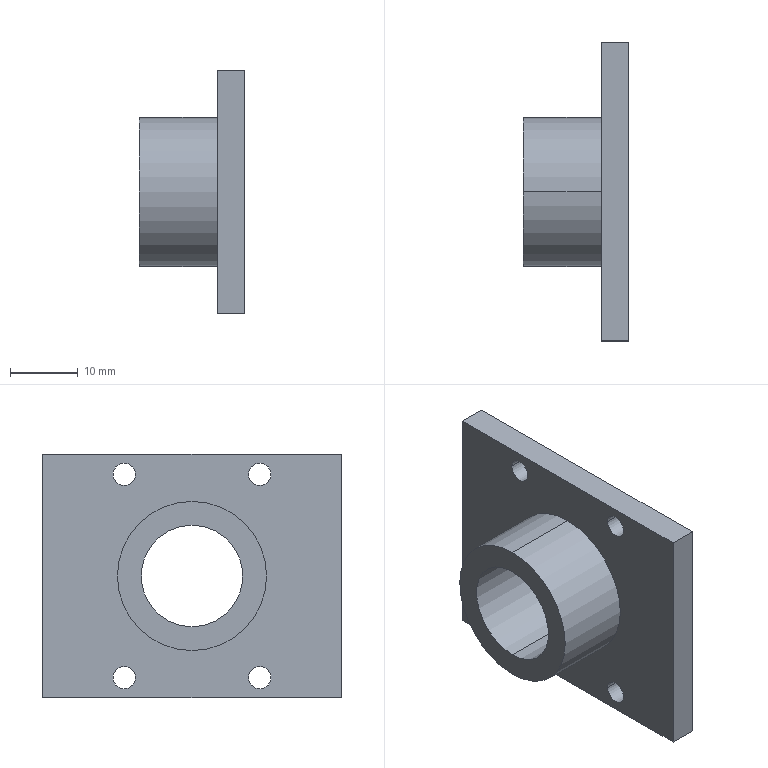Part | SolidWorks | features BaseBody 1 | 1 solid | 19 faces | box 15.5 x 44 x 36 mm | volume 7832 mm3 | cylinder 12 | plane 7 | commonest cylinder face diameters 3.3 x8 15 x2 22 x2
STEP:
#1=CARTESIAN_POINT('',(-2.,-11.65,33.));
#2=VERTEX_POINT('',#1);
#3=CARTESIAN_POINT('',(-2.,-8.35,33.));
#4=VERTEX_POINT('',#3);
#5=CARTESIAN_POINT('',(-2.,-10.,33.));
#6=DIRECTION('',(1.,0.,0.));
#7=DIRECTION('',(0.,1.,0.));
#8=AXIS2_PLACEMENT_3D('',#5,#6,#7);
#9=CIRCLE('',#8,1.65);
#10=EDGE_CURVE('',#2,#4,#9,.T.);
#11=ORIENTED_EDGE('',*,*,#10,.F.);
#12=CARTESIAN_POINT('',(2.,-11.65,33.));
#13=VERTEX_POINT('',#12);
#14=CARTESIAN_POINT('',(-14.2,-11.65,33.));
#15=DIRECTION('',(1.,0.,0.));
#16=VECTOR('',#15,1000.);
#17=LINE('',#14,#16);
#18=EDGE_CURVE('',#2,#13,#17,.T.);
#19=ORIENTED_EDGE('',*,*,#18,.T.);
#20=CARTESIAN_POINT('',(2.,-8.35,33.));
#21=VERTEX_POINT('',#20);
#22=CARTESIAN_POINT('',(2.,-10.,33.));
#23=DIRECTION('',(-1.,0.,0.));
#24=DIRECTION('',(0.,1.,0.));
#25=AXIS2_PLACEMENT_3D('',#22,#23,#24);
#26=CIRCLE('',#25,1.65);
#27=EDGE_CURVE('',#21,#13,#26,.T.);
#28=ORIENTED_EDGE('',*,*,#27,.F.);
#29=CARTESIAN_POINT('',(-14.2,-8.35,33.));
#30=DIRECTION('',(1.,0.,0.));
#31=VECTOR('',#30,1000.);
#32=LINE('',#29,#31);
#33=EDGE_CURVE('',#4,#21,#32,.T.);
#34=ORIENTED_EDGE('',*,*,#33,.F.);
#35=EDGE_LOOP('',(#11,#19,#28,#34));
#36=FACE_OUTER_BOUND('',#35,.T.);
#37=CARTESIAN_POINT('',(-14.2,-10.,33.));
#38=DIRECTION('',(1.,0.,0.));
#39=DIRECTION('',(0.,1.,0.));
#40=AXIS2_PLACEMENT_3D('',#37,#38,#39);
#41=CYLINDRICAL_SURFACE('',#40,1.65);
#42=ADVANCED_FACE('',(#36),#41,.F.);
#43=CARTESIAN_POINT('',(-13.5,0.,25.5));
#44=VERTEX_POINT('',#43);
#45=CARTESIAN_POINT('',(-13.5,0.,10.5));
#46=VERTEX_POINT('',#45);
#47=CARTESIAN_POINT('',(-13.5,0.,18.));
#48=DIRECTION('',(1.,0.,0.));
#49=DIRECTION('',(0.,0.,-1.));
#50=AXIS2_PLACEMENT_3D('',#47,#48,#49);
#51=CIRCLE('',#50,7.5);
#52=EDGE_CURVE('',#44,#46,#51,.T.);
#53=ORIENTED_EDGE('',*,*,#52,.F.);
#54=CARTESIAN_POINT('',(2.,0.,25.5));
#55=VERTEX_POINT('',#54);
#56=CARTESIAN_POINT('',(-3.,0.,25.5));
#57=DIRECTION('',(1.,0.,0.));
#58=VECTOR('',#57,1000.);
#59=LINE('',#56,#58);
#60=EDGE_CURVE('',#44,#55,#59,.T.);
#61=ORIENTED_EDGE('',*,*,#60,.T.);
#62=CARTESIAN_POINT('',(2.,0.,10.5));
#63=VERTEX_POINT('',#62);
#64=CARTESIAN_POINT('',(2.,0.,18.));
#65=DIRECTION('',(-1.,0.,0.));
#66=DIRECTION('',(0.,0.,-1.));
#67=AXIS2_PLACEMENT_3D('',#64,#65,#66);
#68=CIRCLE('',#67,7.5);
#69=EDGE_CURVE('',#63,#55,#68,.T.);
#70=ORIENTED_EDGE('',*,*,#69,.F.);
#71=CARTESIAN_POINT('',(-3.,0.,10.5));
#72=DIRECTION('',(1.,0.,0.));
#73=VECTOR('',#72,1000.);
#74=LINE('',#71,#73);
#75=EDGE_CURVE('',#46,#63,#74,.T.);
#76=ORIENTED_EDGE('',*,*,#75,.F.);
#77=EDGE_LOOP('',(#53,#61,#70,#76));
#78=FACE_OUTER_BOUND('',#77,.T.);
#79=CARTESIAN_POINT('',(-3.,0.,18.));
#80=DIRECTION('',(1.,0.,0.));
#81=DIRECTION('',(0.,0.,-1.));
#82=AXIS2_PLACEMENT_3D('',#79,#80,#81);
#83=CYLINDRICAL_SURFACE('',#82,7.5);
#84=ADVANCED_FACE('',(#78),#83,.F.);
#85=CARTESIAN_POINT('',(-2.,-11.65,3.));
#86=VERTEX_POINT('',#85);
#87=CARTESIAN_POINT('',(-2.,-8.35,3.));
#88=VERTEX_POINT('',#87);
#89=CARTESIAN_POINT('',(-2.,-10.,3.));
#90=DIRECTION('',(1.,0.,0.));
#91=DIRECTION('',(0.,1.,0.));
#92=AXIS2_PLACEMENT_3D('',#89,#90,#91);
#93=CIRCLE('',#92,1.65);
#94=EDGE_CURVE('',#86,#88,#93,.T.);
#95=ORIENTED_EDGE('',*,*,#94,.F.);
#96=CARTESIAN_POINT('',(2.,-11.65,3.));
#97=VERTEX_POINT('',#96);
#98=CARTESIAN_POINT('',(-14.2,-11.65,3.));
#99=DIRECTION('',(1.,0.,0.));
#100=VECTOR('',#99,1000.);
#101=LINE('',#98,#100);
#102=EDGE_CURVE('',#86,#97,#101,.T.);
#103=ORIENTED_EDGE('',*,*,#102,.T.);
#104=CARTESIAN_POINT('',(2.,-8.35,3.));
#105=VERTEX_POINT('',#104);
#106=CARTESIAN_POINT('',(2.,-10.,3.));
#107=DIRECTION('',(-1.,0.,0.));
#108=DIRECTION('',(0.,1.,0.));
#109=AXIS2_PLACEMENT_3D('',#106,#107,#108);
#110=CIRCLE('',#109,1.65);
#111=EDGE_CURVE('',#105,#97,#110,.T.);
#112=ORIENTED_EDGE('',*,*,#111,.F.);
#113=CARTESIAN_POINT('',(-14.2,-8.35,3.));
#114=DIRECTION('',(1.,0.,0.));
#115=VECTOR('',#114,1000.);
#116=LINE('',#113,#115);
#117=EDGE_CURVE('',#88,#105,#116,.T.);
#118=ORIENTED_EDGE('',*,*,#117,.F.);
#119=EDGE_LOOP('',(#95,#103,#112,#118));
#120=FACE_OUTER_BOUND('',#119,.T.);
#121=CARTESIAN_POINT('',(-14.2,-10.,3.));
#122=DIRECTION('',(1.,0.,0.));
#123=DIRECTION('',(0.,1.,0.));
#124=AXIS2_PLACEMENT_3D('',#121,#122,#123);
#125=CYLINDRICAL_SURFACE('',#124,1.65);
#126=ADVANCED_FACE('',(#120),#125,.F.);
#127=CARTESIAN_POINT('',(-2.,8.35,33.));
#128=VERTEX_POINT('',#127);
#129=CARTESIAN_POINT('',(-2.,11.65,33.));
#130=VERTEX_POINT('',#129);
#131=CARTESIAN_POINT('',(-2.,10.,33.));
#132=DIRECTION('',(1.,0.,0.));
#133=DIRECTION('',(0.,1.,0.));
#134=AXIS2_PLACEMENT_3D('',#131,#132,#133);
#135=CIRCLE('',#134,1.65);
#136=EDGE_CURVE('',#128,#130,#135,.T.);
#137=ORIENTED_EDGE('',*,*,#136,.F.);
#138=CARTESIAN_POINT('',(2.,8.35,33.));
#139=VERTEX_POINT('',#138);
#140=CARTESIAN_POINT('',(-14.2,8.35,33.));
#141=DIRECTION('',(1.,0.,0.));
#142=VECTOR('',#141,1000.);
#143=LINE('',#140,#142);
#144=EDGE_CURVE('',#128,#139,#143,.T.);
#145=ORIENTED_EDGE('',*,*,#144,.T.);
#146=CARTESIAN_POINT('',(2.,11.65,33.));
#147=VERTEX_POINT('',#146);
#148=CARTESIAN_POINT('',(2.,10.,33.));
#149=DIRECTION('',(-1.,0.,0.));
#150=DIRECTION('',(0.,1.,0.));
#151=AXIS2_PLACEMENT_3D('',#148,#149,#150);
#152=CIRCLE('',#151,1.65);
#153=EDGE_CURVE('',#147,#139,#152,.T.);
#154=ORIENTED_EDGE('',*,*,#153,.F.);
#155=CARTESIAN_POINT('',(-14.2,11.65,33.));
#156=DIRECTION('',(1.,0.,0.));
#157=VECTOR('',#156,1000.);
#158=LINE('',#155,#157);
#159=EDGE_CURVE('',#130,#147,#158,.T.);
#160=ORIENTED_EDGE('',*,*,#159,.F.);
#161=EDGE_LOOP('',(#137,#145,#154,#160));
#162=FACE_OUTER_BOUND('',#161,.T.);
#163=CARTESIAN_POINT('',(-14.2,10.,33.));
#164=DIRECTION('',(1.,0.,0.));
#165=DIRECTION('',(0.,1.,0.));
#166=AXIS2_PLACEMENT_3D('',#163,#164,#165);
#167=CYLINDRICAL_SURFACE('',#166,1.65);
#168=ADVANCED_FACE('',(#162),#167,.F.);
#169=CARTESIAN_POINT('',(-2.,8.35,3.));
#170=VERTEX_POINT('',#169);
#171=CARTESIAN_POINT('',(-2.,11.65,3.));
#172=VERTEX_POINT('',#171);
#173=CARTESIAN_POINT('',(-2.,10.,3.));
#174=DIRECTION('',(1.,0.,0.));
#175=DIRECTION('',(0.,1.,0.));
#176=AXIS2_PLACEMENT_3D('',#173,#174,#175);
#177=CIRCLE('',#176,1.65);
#178=EDGE_CURVE('',#170,#172,#177,.T.);
#179=ORIENTED_EDGE('',*,*,#178,.F.);
#180=CARTESIAN_POINT('',(2.,8.35,3.));
#181=VERTEX_POINT('',#180);
#182=CARTESIAN_POINT('',(-14.2,8.35,3.));
#183=DIRECTION('',(1.,0.,0.));
#184=VECTOR('',#183,1000.);
#185=LINE('',#182,#184);
#186=EDGE_CURVE('',#170,#181,#185,.T.);
#187=ORIENTED_EDGE('',*,*,#186,.T.);
#188=CARTESIAN_POINT('',(2.,11.65,3.));
#189=VERTEX_POINT('',#188);
#190=CARTESIAN_POINT('',(2.,10.,3.));
#191=DIRECTION('',(-1.,0.,0.));
#192=DIRECTION('',(0.,1.,0.));
#193=AXIS2_PLACEMENT_3D('',#190,#191,#192);
#194=CIRCLE('',#193,1.65);
#195=EDGE_CURVE('',#189,#181,#194,.T.);
#196=ORIENTED_EDGE('',*,*,#195,.F.);
#197=CARTESIAN_POINT('',(-14.2,11.65,3.));
#198=DIRECTION('',(1.,0.,0.));
#199=VECTOR('',#198,1000.);
#200=LINE('',#197,#199);
#201=EDGE_CURVE('',#172,#189,#200,.T.);
#202=ORIENTED_EDGE('',*,*,#201,.F.);
#203=EDGE_LOOP('',(#179,#187,#196,#202));
#204=FACE_OUTER_BOUND('',#203,.T.);
#205=CARTESIAN_POINT('',(-14.2,10.,3.));
#206=DIRECTION('',(1.,0.,0.));
#207=DIRECTION('',(0.,1.,0.));
#208=AXIS2_PLACEMENT_3D('',#205,#206,#207);
#209=CYLINDRICAL_SURFACE('',#208,1.65);
#210=ADVANCED_FACE('',(#204),#209,.F.);
#211=CARTESIAN_POINT('',(-13.5,0.,7.));
#212=VERTEX_POINT('',#211);
#213=CARTESIAN_POINT('',(-13.5,0.,29.));
#214=VERTEX_POINT('',#213);
#215=CARTESIAN_POINT('',(-13.5,0.,18.));
#216=DIRECTION('',(1.,0.,0.));
#217=DIRECTION('',(0.,0.,-1.));
#218=AXIS2_PLACEMENT_3D('',#215,#216,#217);
#219=CIRCLE('',#218,11.);
#220=EDGE_CURVE('',#212,#214,#219,.T.);
#221=ORIENTED_EDGE('',*,*,#220,.T.);
#222=CARTESIAN_POINT('',(-2.,0.,29.));
#223=VERTEX_POINT('',#222);
#224=CARTESIAN_POINT('',(-13.5,0.,29.));
#225=DIRECTION('',(1.,0.,0.));
#226=VECTOR('',#225,1000.);
#227=LINE('',#224,#226);
#228=EDGE_CURVE('',#214,#223,#227,.T.);
#229=ORIENTED_EDGE('',*,*,#228,.T.);
#230=CARTESIAN_POINT('',(-2.,0.,7.));
#231=VERTEX_POINT('',#230);
#232=CARTESIAN_POINT('',(-2.,0.,18.));
#233=DIRECTION('',(-1.,0.,0.));
#234=DIRECTION('',(0.,0.,-1.));
#235=AXIS2_PLACEMENT_3D('',#232,#233,#234);
#236=CIRCLE('',#235,11.);
#237=EDGE_CURVE('',#223,#231,#236,.T.);
#238=ORIENTED_EDGE('',*,*,#237,.T.);
#239=CARTESIAN_POINT('',(-13.5,0.,7.));
#240=DIRECTION('',(1.,0.,0.));
#241=VECTOR('',#240,1000.);
#242=LINE('',#239,#241);
#243=EDGE_CURVE('',#212,#231,#242,.T.);
#244=ORIENTED_EDGE('',*,*,#243,.F.);
#245=EDGE_LOOP('',(#221,#229,#238,#244));
#246=FACE_OUTER_BOUND('',#245,.T.);
#247=CARTESIAN_POINT('',(-13.5,0.,18.));
#248=DIRECTION('',(1.,0.,0.));
#249=DIRECTION('',(0.,0.,-1.));
#250=AXIS2_PLACEMENT_3D('',#247,#248,#249);
#251=CYLINDRICAL_SURFACE('',#250,11.);
#252=ADVANCED_FACE('',(#246),#251,.T.);
#253=ORIENTED_EDGE('',*,*,#27,.T.);
#254=CARTESIAN_POINT('',(2.,-10.,33.));
#255=DIRECTION('',(-1.,0.,0.));
#256=DIRECTION('',(0.,1.,0.));
#257=AXIS2_PLACEMENT_3D('',#254,#255,#256);
#258=CIRCLE('',#257,1.65);
#259=EDGE_CURVE('',#13,#21,#258,.T.);
#260=ORIENTED_EDGE('',*,*,#259,.T.);
#261=EDGE_LOOP('',(#253,#260));
#262=FACE_BOUND('',#261,.T.);
#263=ORIENTED_EDGE('',*,*,#69,.T.);
#264=CARTESIAN_POINT('',(2.,0.,18.));
#265=DIRECTION('',(-1.,0.,0.));
#266=DIRECTION('',(0.,0.,-1.));
#267=AXIS2_PLACEMENT_3D('',#264,#265,#266);
#268=CIRCLE('',#267,7.5);
#269=EDGE_CURVE('',#55,#63,#268,.T.);
#270=ORIENTED_EDGE('',*,*,#269,.T.);
#271=EDGE_LOOP('',(#263,#270));
#272=FACE_BOUND('',#271,.T.);
#273=ORIENTED_EDGE('',*,*,#111,.T.);
#274=CARTESIAN_POINT('',(2.,-10.,3.));
#275=DIRECTION('',(-1.,0.,0.));
#276=DIRECTION('',(0.,1.,0.));
#277=AXIS2_PLACEMENT_3D('',#274,#275,#276);
#278=CIRCLE('',#277,1.65);
#279=EDGE_CURVE('',#97,#105,#278,.T.);
#280=ORIENTED_EDGE('',*,*,#279,.T.);
#281=EDGE_LOOP('',(#273,#280));
#282=FACE_BOUND('',#281,.T.);
#283=ORIENTED_EDGE('',*,*,#153,.T.);
#284=CARTESIAN_POINT('',(2.,10.,33.));
#285=DIRECTION('',(-1.,0.,0.));
#286=DIRECTION('',(0.,1.,0.));
#287=AXIS2_PLACEMENT_3D('',#284,#285,#286);
#288=CIRCLE('',#287,1.65);
#289=EDGE_CURVE('',#139,#147,#288,.T.);
#290=ORIENTED_EDGE('',*,*,#289,.T.);
#291=EDGE_LOOP('',(#283,#290));
#292=FACE_BOUND('',#291,.T.);
#293=ORIENTED_EDGE('',*,*,#195,.T.);
#294=CARTESIAN_POINT('',(2.,10.,3.));
#295=DIRECTION('',(-1.,0.,0.));
#296=DIRECTION('',(0.,1.,0.));
#297=AXIS2_PLACEMENT_3D('',#294,#295,#296);
#298=CIRCLE('',#297,1.65);
#299=EDGE_CURVE('',#181,#189,#298,.T.);
#300=ORIENTED_EDGE('',*,*,#299,.T.);
#301=EDGE_LOOP('',(#293,#300));
#302=FACE_BOUND('',#301,.T.);
#303=CARTESIAN_POINT('',(2.,22.,0.));
#304=VERTEX_POINT('',#303);
#305=CARTESIAN_POINT('',(2.,22.,36.));
#306=VERTEX_POINT('',#305);
#307=CARTESIAN_POINT('',(2.,22.,0.));
#308=DIRECTION('',(0.,0.,1.));
#309=VECTOR('',#308,1000.);
#310=LINE('',#307,#309);
#311=EDGE_CURVE('',#304,#306,#310,.T.);
#312=ORIENTED_EDGE('',*,*,#311,.T.);
#313=CARTESIAN_POINT('',(2.,-22.,36.));
#314=VERTEX_POINT('',#313);
#315=CARTESIAN_POINT('',(2.,-22.,36.));
#316=DIRECTION('',(0.,-1.,0.));
#317=VECTOR('',#316,1000.);
#318=LINE('',#315,#317);
#319=EDGE_CURVE('',#306,#314,#318,.T.);
#320=ORIENTED_EDGE('',*,*,#319,.T.);
#321=CARTESIAN_POINT('',(2.,-22.,0.));
#322=VERTEX_POINT('',#321);
#323=CARTESIAN_POINT('',(2.,-22.,0.));
#324=DIRECTION('',(0.,0.,-1.));
#325=VECTOR('',#324,1000.);
#326=LINE('',#323,#325);
#327=EDGE_CURVE('',#314,#322,#326,.T.);
#328=ORIENTED_EDGE('',*,*,#327,.T.);
#329=CARTESIAN_POINT('',(2.,-22.,0.));
#330=DIRECTION('',(0.,1.,0.));
#331=VECTOR('',#330,1000.);
#332=LINE('',#329,#331);
#333=EDGE_CURVE('',#322,#304,#332,.T.);
#334=ORIENTED_EDGE('',*,*,#333,.T.);
#335=EDGE_LOOP('',(#312,#320,#328,#334));
#336=FACE_OUTER_BOUND('',#335,.T.);
#337=CARTESIAN_POINT('',(2.,-22.,0.));
#338=DIRECTION('',(1.,0.,0.));
#339=DIRECTION('',(0.,0.,-1.));
#340=AXIS2_PLACEMENT_3D('',#337,#338,#339);
#341=PLANE('',#340);
#342=ADVANCED_FACE('',(#262,#272,#282,#292,#302,#336),#341,.T.);
#343=ORIENTED_EDGE('',*,*,#18,.F.);
#344=CARTESIAN_POINT('',(-2.,-10.,33.));
#345=DIRECTION('',(1.,0.,0.));
#346=DIRECTION('',(0.,1.,0.));
#347=AXIS2_PLACEMENT_3D('',#344,#345,#346);
#348=CIRCLE('',#347,1.65);
#349=EDGE_CURVE('',#4,#2,#348,.T.);
#350=ORIENTED_EDGE('',*,*,#349,.F.);
#351=ORIENTED_EDGE('',*,*,#33,.T.);
#352=ORIENTED_EDGE('',*,*,#259,.F.);
#353=EDGE_LOOP('',(#343,#350,#351,#352));
#354=FACE_OUTER_BOUND('',#353,.T.);
#355=CARTESIAN_POINT('',(-14.2,-10.,33.));
#356=DIRECTION('',(1.,0.,0.));
#357=DIRECTION('',(0.,1.,0.));
#358=AXIS2_PLACEMENT_3D('',#355,#356,#357);
#359=CYLINDRICAL_SURFACE('',#358,1.65);
#360=ADVANCED_FACE('',(#354),#359,.F.);
#361=ORIENTED_EDGE('',*,*,#60,.F.);
#362=CARTESIAN_POINT('',(-13.5,0.,18.));
#363=DIRECTION('',(1.,0.,0.));
#364=DIRECTION('',(0.,0.,-1.));
#365=AXIS2_PLACEMENT_3D('',#362,#363,#364);
#366=CIRCLE('',#365,7.5);
#367=EDGE_CURVE('',#46,#44,#366,.T.);
#368=ORIENTED_EDGE('',*,*,#367,.F.);
#369=ORIENTED_EDGE('',*,*,#75,.T.);
#370=ORIENTED_EDGE('',*,*,#269,.F.);
#371=EDGE_LOOP('',(#361,#368,#369,#370));
#372=FACE_OUTER_BOUND('',#371,.T.);
#373=CARTESIAN_POINT('',(-3.,0.,18.));
#374=DIRECTION('',(1.,0.,0.));
#375=DIRECTION('',(0.,0.,-1.));
#376=AXIS2_PLACEMENT_3D('',#373,#374,#375);
#377=CYLINDRICAL_SURFACE('',#376,7.5);
#378=ADVANCED_FACE('',(#372),#377,.F.);
#379=ORIENTED_EDGE('',*,*,#102,.F.);
#380=CARTESIAN_POINT('',(-2.,-10.,3.));
#381=DIRECTION('',(1.,0.,0.));
#382=DIRECTION('',(0.,1.,0.));
#383=AXIS2_PLACEMENT_3D('',#380,#381,#382);
#384=CIRCLE('',#383,1.65);
#385=EDGE_CURVE('',#88,#86,#384,.T.);
#386=ORIENTED_EDGE('',*,*,#385,.F.);
#387=ORIENTED_EDGE('',*,*,#117,.T.);
#388=ORIENTED_EDGE('',*,*,#279,.F.);
#389=EDGE_LOOP('',(#379,#386,#387,#388));
#390=FACE_OUTER_BOUND('',#389,.T.);
#391=CARTESIAN_POINT('',(-14.2,-10.,3.));
#392=DIRECTION('',(1.,0.,0.));
#393=DIRECTION('',(0.,1.,0.));
#394=AXIS2_PLACEMENT_3D('',#391,#392,#393);
#395=CYLINDRICAL_SURFACE('',#394,1.65);
#396=ADVANCED_FACE('',(#390),#395,.F.);
#397=ORIENTED_EDGE('',*,*,#144,.F.);
#398=CARTESIAN_POINT('',(-2.,10.,33.));
#399=DIRECTION('',(1.,0.,0.));
#400=DIRECTION('',(0.,1.,0.));
#401=AXIS2_PLACEMENT_3D('',#398,#399,#400);
#402=CIRCLE('',#401,1.65);
#403=EDGE_CURVE('',#130,#128,#402,.T.);
#404=ORIENTED_EDGE('',*,*,#403,.F.);
#405=ORIENTED_EDGE('',*,*,#159,.T.);
#406=ORIENTED_EDGE('',*,*,#289,.F.);
#407=EDGE_LOOP('',(#397,#404,#405,#406));
#408=FACE_OUTER_BOUND('',#407,.T.);
#409=CARTESIAN_POINT('',(-14.2,10.,33.));
#410=DIRECTION('',(1.,0.,0.));
#411=DIRECTION('',(0.,1.,0.));
#412=AXIS2_PLACEMENT_3D('',#409,#410,#411);
#413=CYLINDRICAL_SURFACE('',#412,1.65);
#414=ADVANCED_FACE('',(#408),#413,.F.);
#415=ORIENTED_EDGE('',*,*,#186,.F.);
#416=CARTESIAN_POINT('',(-2.,10.,3.));
#417=DIRECTION('',(1.,0.,0.));
#418=DIRECTION('',(0.,1.,0.));
#419=AXIS2_PLACEMENT_3D('',#416,#417,#418);
#420=CIRCLE('',#419,1.65);
#421=EDGE_CURVE('',#172,#170,#420,.T.);
#422=ORIENTED_EDGE('',*,*,#421,.F.);
#423=ORIENTED_EDGE('',*,*,#201,.T.);
#424=ORIENTED_EDGE('',*,*,#299,.F.);
#425=EDGE_LOOP('',(#415,#422,#423,#424));
#426=FACE_OUTER_BOUND('',#425,.T.);
#427=CARTESIAN_POINT('',(-14.2,10.,3.));
#428=DIRECTION('',(1.,0.,0.));
#429=DIRECTION('',(0.,1.,0.));
#430=AXIS2_PLACEMENT_3D('',#427,#428,#429);
#431=CYLINDRICAL_SURFACE('',#430,1.65);
#432=ADVANCED_FACE('',(#426),#431,.F.);
#433=ORIENTED_EDGE('',*,*,#319,.F.);
#434=CARTESIAN_POINT('',(-2.,22.,36.));
#435=VERTEX_POINT('',#434);
#436=CARTESIAN_POINT('',(-2.,22.,36.));
#437=DIRECTION('',(-1.,0.,0.));
#438=VECTOR('',#437,1000.);
#439=LINE('',#436,#438);
#440=EDGE_CURVE('',#306,#435,#439,.T.);
#441=ORIENTED_EDGE('',*,*,#440,.T.);
#442=CARTESIAN_POINT('',(-2.,-22.,36.));
#443=VERTEX_POINT('',#442);
#444=CARTESIAN_POINT('',(-2.,-22.,36.));
#445=DIRECTION('',(0.,-1.,0.));
#446=VECTOR('',#445,1000.);
#447=LINE('',#444,#446);
#448=EDGE_CURVE('',#435,#443,#447,.T.);
#449=ORIENTED_EDGE('',*,*,#448,.T.);
#450=CARTESIAN_POINT('',(-2.,-22.,36.));
#451=DIRECTION('',(1.,0.,0.));
#452=VECTOR('',#451,1000.);
#453=LINE('',#450,#452);
#454=EDGE_CURVE('',#443,#314,#453,.T.);
#455=ORIENTED_EDGE('',*,*,#454,.T.);
#456=EDGE_LOOP('',(#433,#441,#449,#455));
#457=FACE_OUTER_BOUND('',#456,.T.);
#458=CARTESIAN_POINT('',(-2.,-22.,36.));
#459=DIRECTION('',(0.,0.,1.));
#460=DIRECTION('',(1.,0.,0.));
#461=AXIS2_PLACEMENT_3D('',#458,#459,#460);
#462=PLANE('',#461);
#463=ADVANCED_FACE('',(#457),#462,.T.);
#464=ORIENTED_EDGE('',*,*,#440,.F.);
#465=ORIENTED_EDGE('',*,*,#311,.F.);
#466=CARTESIAN_POINT('',(-2.,22.,0.));
#467=VERTEX_POINT('',#466);
#468=CARTESIAN_POINT('',(-2.,22.,0.));
#469=DIRECTION('',(-1.,0.,0.));
#470=VECTOR('',#469,1000.);
#471=LINE('',#468,#470);
#472=EDGE_CURVE('',#304,#467,#471,.T.);
#473=ORIENTED_EDGE('',*,*,#472,.T.);
#474=CARTESIAN_POINT('',(-2.,22.,0.));
#475=DIRECTION('',(0.,0.,1.));
#476=VECTOR('',#475,1000.);
#477=LINE('',#474,#476);
#478=EDGE_CURVE('',#467,#435,#477,.T.);
#479=ORIENTED_EDGE('',*,*,#478,.T.);
#480=EDGE_LOOP('',(#464,#465,#473,#479));
#481=FACE_OUTER_BOUND('',#480,.T.);
#482=CARTESIAN_POINT('',(-2.,22.,0.));
#483=DIRECTION('',(0.,1.,0.));
#484=DIRECTION('',(0.,0.,1.));
#485=AXIS2_PLACEMENT_3D('',#482,#483,#484);
#486=PLANE('',#485);
#487=ADVANCED_FACE('',(#481),#486,.T.);
#488=ORIENTED_EDGE('',*,*,#333,.F.);
#489=CARTESIAN_POINT('',(-2.,-22.,0.));
#490=VERTEX_POINT('',#489);
#491=CARTESIAN_POINT('',(-2.,-22.,0.));
#492=DIRECTION('',(1.,0.,0.));
#493=VECTOR('',#492,1000.);
#494=LINE('',#491,#493);
#495=EDGE_CURVE('',#490,#322,#494,.T.);
#496=ORIENTED_EDGE('',*,*,#495,.F.);
#497=CARTESIAN_POINT('',(-2.,-22.,0.));
#498=DIRECTION('',(0.,-1.,0.));
#499=VECTOR('',#498,1000.);
#500=LINE('',#497,#499);
#501=EDGE_CURVE('',#467,#490,#500,.T.);
#502=ORIENTED_EDGE('',*,*,#501,.F.);
#503=ORIENTED_EDGE('',*,*,#472,.F.);
#504=EDGE_LOOP('',(#488,#496,#502,#503));
#505=FACE_OUTER_BOUND('',#504,.T.);
#506=CARTESIAN_POINT('',(-2.,-22.,0.));
#507=DIRECTION('',(0.,0.,1.));
#508=DIRECTION('',(1.,0.,0.));
#509=AXIS2_PLACEMENT_3D('',#506,#507,#508);
#510=PLANE('',#509);
#511=ADVANCED_FACE('',(#505),#510,.F.);
#512=ORIENTED_EDGE('',*,*,#454,.F.);
#513=CARTESIAN_POINT('',(-2.,-22.,0.));
#514=DIRECTION('',(0.,0.,1.));
#515=VECTOR('',#514,1000.);
#516=LINE('',#513,#515);
#517=EDGE_CURVE('',#490,#443,#516,.T.);
#518=ORIENTED_EDGE('',*,*,#517,.F.);
#519=ORIENTED_EDGE('',*,*,#495,.T.);
#520=ORIENTED_EDGE('',*,*,#327,.F.);
#521=EDGE_LOOP('',(#512,#518,#519,#520));
#522=FACE_OUTER_BOUND('',#521,.T.);
#523=CARTESIAN_POINT('',(-2.,-22.,0.));
#524=DIRECTION('',(0.,1.,0.));
#525=DIRECTION('',(0.,0.,1.));
#526=AXIS2_PLACEMENT_3D('',#523,#524,#525);
#527=PLANE('',#526);
#528=ADVANCED_FACE('',(#522),#527,.F.);
#529=ORIENTED_EDGE('',*,*,#349,.T.);
#530=ORIENTED_EDGE('',*,*,#10,.T.);
#531=EDGE_LOOP('',(#529,#530));
#532=FACE_BOUND('',#531,.T.);
#533=CARTESIAN_POINT('',(-2.,0.,18.));
#534=DIRECTION('',(-1.,0.,0.));
#535=DIRECTION('',(0.,0.,-1.));
#536=AXIS2_PLACEMENT_3D('',#533,#534,#535);
#537=CIRCLE('',#536,11.);
#538=EDGE_CURVE('',#231,#223,#537,.T.);
#539=ORIENTED_EDGE('',*,*,#538,.F.);
#540=ORIENTED_EDGE('',*,*,#237,.F.);
#541=EDGE_LOOP('',(#539,#540));
#542=FACE_BOUND('',#541,.T.);
#543=ORIENTED_EDGE('',*,*,#385,.T.);
#544=ORIENTED_EDGE('',*,*,#94,.T.);
#545=EDGE_LOOP('',(#543,#544));
#546=FACE_BOUND('',#545,.T.);
#547=ORIENTED_EDGE('',*,*,#403,.T.);
#548=ORIENTED_EDGE('',*,*,#136,.T.);
#549=EDGE_LOOP('',(#547,#548));
#550=FACE_BOUND('',#549,.T.);
#551=ORIENTED_EDGE('',*,*,#421,.T.);
#552=ORIENTED_EDGE('',*,*,#178,.T.);
#553=EDGE_LOOP('',(#551,#552));
#554=FACE_BOUND('',#553,.T.);
#555=ORIENTED_EDGE('',*,*,#478,.F.);
#556=ORIENTED_EDGE('',*,*,#501,.T.);
#557=ORIENTED_EDGE('',*,*,#517,.T.);
#558=ORIENTED_EDGE('',*,*,#448,.F.);
#559=EDGE_LOOP('',(#555,#556,#557,#558));
#560=FACE_OUTER_BOUND('',#559,.T.);
#561=CARTESIAN_POINT('',(-2.,-22.,0.));
#562=DIRECTION('',(1.,0.,0.));
#563=DIRECTION('',(0.,0.,-1.));
#564=AXIS2_PLACEMENT_3D('',#561,#562,#563);
#565=PLANE('',#564);
#566=ADVANCED_FACE('',(#532,#542,#546,#550,#554,#560),#565,.F.);
#567=ORIENTED_EDGE('',*,*,#367,.T.);
#568=ORIENTED_EDGE('',*,*,#52,.T.);
#569=EDGE_LOOP('',(#567,#568));
#570=FACE_BOUND('',#569,.T.);
#571=ORIENTED_EDGE('',*,*,#220,.F.);
#572=CARTESIAN_POINT('',(-13.5,0.,18.));
#573=DIRECTION('',(1.,0.,0.));
#574=DIRECTION('',(0.,0.,-1.));
#575=AXIS2_PLACEMENT_3D('',#572,#573,#574);
#576=CIRCLE('',#575,11.);
#577=EDGE_CURVE('',#214,#212,#576,.T.);
#578=ORIENTED_EDGE('',*,*,#577,.F.);
#579=EDGE_LOOP('',(#571,#578));
#580=FACE_OUTER_BOUND('',#579,.T.);
#581=CARTESIAN_POINT('',(-13.5,0.,18.));
#582=DIRECTION('',(1.,0.,0.));
#583=DIRECTION('',(0.,0.,-1.));
#584=AXIS2_PLACEMENT_3D('',#581,#582,#583);
#585=PLANE('',#584);
#586=ADVANCED_FACE('',(#570,#580),#585,.F.);
#587=ORIENTED_EDGE('',*,*,#228,.F.);
#588=ORIENTED_EDGE('',*,*,#577,.T.);
#589=ORIENTED_EDGE('',*,*,#243,.T.);
#590=ORIENTED_EDGE('',*,*,#538,.T.);
#591=EDGE_LOOP('',(#587,#588,#589,#590));
#592=FACE_OUTER_BOUND('',#591,.T.);
#593=CARTESIAN_POINT('',(-13.5,0.,18.));
#594=DIRECTION('',(1.,0.,0.));
#595=DIRECTION('',(0.,0.,-1.));
#596=AXIS2_PLACEMENT_3D('',#593,#594,#595);
#597=CYLINDRICAL_SURFACE('',#596,11.);
#598=ADVANCED_FACE('',(#592),#597,.T.);
#599=CLOSED_SHELL('',(#42,#84,#126,#168,#210,#252,#342,#360,#378,#396,#414,#432,#463,#487,#511,#528,#566,#586,#598));
#600=MANIFOLD_SOLID_BREP('',#599);
#601=CARTESIAN_POINT('',(0.,0.,0.));
#602=DIRECTION('',(0.,0.,1.));
#603=DIRECTION('',(1.,0.,0.));
#604=AXIS2_PLACEMENT_3D('',#601,#602,#603);
#605=(LENGTH_UNIT()NAMED_UNIT(*)SI_UNIT(.MILLI.,.METRE.));
#606=UNCERTAINTY_MEASURE_WITH_UNIT(LENGTH_MEASURE(0.00001),#605,'','');
#607=(NAMED_UNIT(*)PLANE_ANGLE_UNIT()SI_UNIT($,.RADIAN.));
#608=(NAMED_UNIT(*)SI_UNIT($,.STERADIAN.)SOLID_ANGLE_UNIT());
#609=(GEOMETRIC_REPRESENTATION_CONTEXT(3)GLOBAL_UNCERTAINTY_ASSIGNED_CONTEXT((#606))GLOBAL_UNIT_ASSIGNED_CONTEXT((#605,#607,#608))REPRESENTATION_CONTEXT('',''));
#610=ADVANCED_BREP_SHAPE_REPRESENTATION('',(#600,#604),#609);